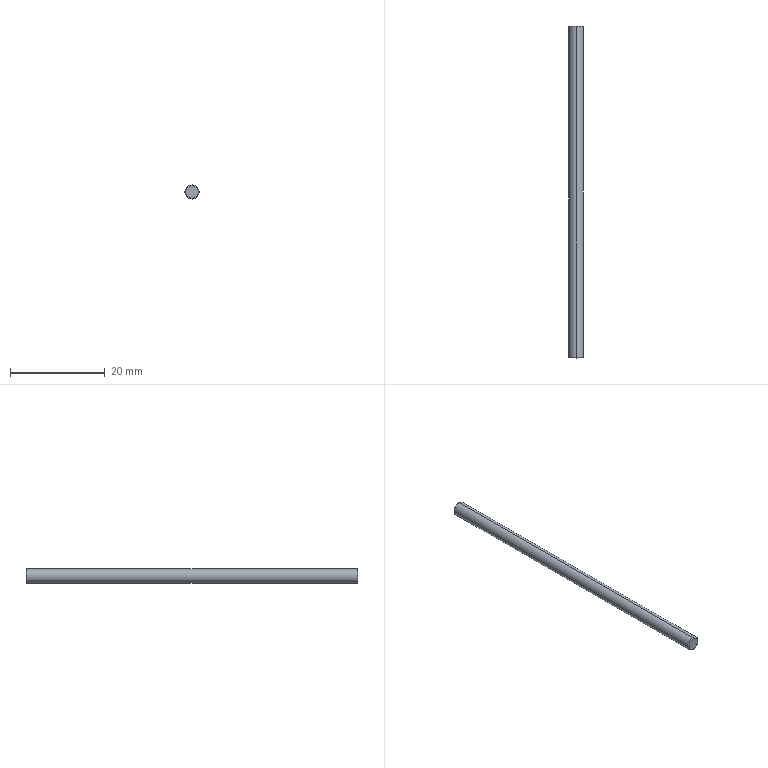Part | SolidWorks | features Extrusion 1, Fillet 1 | 1 solid | 8 faces | box 3 x 70 x 3 mm | volume 494.644 mm3 | torus 4 | cylinder 2 | plane 2 | commonest cylinder face diameters 3 x2
STEP:
#1=CARTESIAN_POINT('',(0.,69.8,-1.5));
#2=VERTEX_POINT('',#1);
#3=CARTESIAN_POINT('',(0.,69.8,1.5));
#4=VERTEX_POINT('',#3);
#5=CARTESIAN_POINT('',(0.,69.8,0.));
#6=DIRECTION('',(0.,-1.,0.));
#7=DIRECTION('',(0.,0.,1.));
#8=AXIS2_PLACEMENT_3D('',#5,#6,#7);
#9=CIRCLE('',#8,1.5);
#10=EDGE_CURVE('',#2,#4,#9,.T.);
#11=ORIENTED_EDGE('',*,*,#10,.F.);
#12=CARTESIAN_POINT('',(0.,70.,-1.3));
#13=VERTEX_POINT('',#12);
#14=CARTESIAN_POINT('',(0.,69.8,-1.3));
#15=DIRECTION('',(1.,0.,0.));
#16=DIRECTION('',(0.,0.,-1.));
#17=AXIS2_PLACEMENT_3D('',#14,#15,#16);
#18=CIRCLE('',#17,0.2);
#19=EDGE_CURVE('',#2,#13,#18,.T.);
#20=ORIENTED_EDGE('',*,*,#19,.T.);
#21=CARTESIAN_POINT('',(0.,70.,1.3));
#22=VERTEX_POINT('',#21);
#23=CARTESIAN_POINT('',(0.,70.,0.));
#24=DIRECTION('',(0.,1.,0.));
#25=DIRECTION('',(0.,0.,1.));
#26=AXIS2_PLACEMENT_3D('',#23,#24,#25);
#27=CIRCLE('',#26,1.3);
#28=EDGE_CURVE('',#22,#13,#27,.T.);
#29=ORIENTED_EDGE('',*,*,#28,.F.);
#30=CARTESIAN_POINT('',(0.,69.8,1.3));
#31=DIRECTION('',(-1.,0.,0.));
#32=DIRECTION('',(0.,0.,1.));
#33=AXIS2_PLACEMENT_3D('',#30,#31,#32);
#34=CIRCLE('',#33,0.2);
#35=EDGE_CURVE('',#4,#22,#34,.T.);
#36=ORIENTED_EDGE('',*,*,#35,.F.);
#37=EDGE_LOOP('',(#11,#20,#29,#36));
#38=FACE_OUTER_BOUND('',#37,.T.);
#39=CARTESIAN_POINT('',(0.,69.8,0.));
#40=DIRECTION('',(0.,1.,0.));
#41=DIRECTION('',(0.,0.,1.));
#42=AXIS2_PLACEMENT_3D('',#39,#40,#41);
#43=TOROIDAL_SURFACE('',#42,1.3,0.2);
#44=ADVANCED_FACE('',(#38),#43,.T.);
#45=CARTESIAN_POINT('',(0.,0.,-1.3));
#46=VERTEX_POINT('',#45);
#47=CARTESIAN_POINT('',(0.,0.,1.3));
#48=VERTEX_POINT('',#47);
#49=CARTESIAN_POINT('',(0.,0.,0.));
#50=DIRECTION('',(0.,-1.,0.));
#51=DIRECTION('',(0.,0.,1.));
#52=AXIS2_PLACEMENT_3D('',#49,#50,#51);
#53=CIRCLE('',#52,1.3);
#54=EDGE_CURVE('',#46,#48,#53,.T.);
#55=ORIENTED_EDGE('',*,*,#54,.F.);
#56=CARTESIAN_POINT('',(0.,0.2,-1.5));
#57=VERTEX_POINT('',#56);
#58=CARTESIAN_POINT('',(0.,0.2,-1.3));
#59=DIRECTION('',(1.,0.,0.));
#60=DIRECTION('',(0.,0.,-1.));
#61=AXIS2_PLACEMENT_3D('',#58,#59,#60);
#62=CIRCLE('',#61,0.2);
#63=EDGE_CURVE('',#46,#57,#62,.T.);
#64=ORIENTED_EDGE('',*,*,#63,.T.);
#65=CARTESIAN_POINT('',(0.,0.2,1.5));
#66=VERTEX_POINT('',#65);
#67=CARTESIAN_POINT('',(0.,0.2,0.));
#68=DIRECTION('',(0.,1.,0.));
#69=DIRECTION('',(0.,0.,1.));
#70=AXIS2_PLACEMENT_3D('',#67,#68,#69);
#71=CIRCLE('',#70,1.5);
#72=EDGE_CURVE('',#66,#57,#71,.T.);
#73=ORIENTED_EDGE('',*,*,#72,.F.);
#74=CARTESIAN_POINT('',(0.,0.2,1.3));
#75=DIRECTION('',(-1.,0.,0.));
#76=DIRECTION('',(0.,0.,1.));
#77=AXIS2_PLACEMENT_3D('',#74,#75,#76);
#78=CIRCLE('',#77,0.2);
#79=EDGE_CURVE('',#48,#66,#78,.T.);
#80=ORIENTED_EDGE('',*,*,#79,.F.);
#81=EDGE_LOOP('',(#55,#64,#73,#80));
#82=FACE_OUTER_BOUND('',#81,.T.);
#83=CARTESIAN_POINT('',(0.,0.2,0.));
#84=DIRECTION('',(0.,1.,0.));
#85=DIRECTION('',(0.,0.,1.));
#86=AXIS2_PLACEMENT_3D('',#83,#84,#85);
#87=TOROIDAL_SURFACE('',#86,1.3,0.2);
#88=ADVANCED_FACE('',(#82),#87,.T.);
#89=ORIENTED_EDGE('',*,*,#10,.T.);
#90=CARTESIAN_POINT('',(0.,70.,1.5));
#91=DIRECTION('',(0.,-1.,0.));
#92=VECTOR('',#91,1000.);
#93=LINE('',#90,#92);
#94=EDGE_CURVE('',#4,#66,#93,.T.);
#95=ORIENTED_EDGE('',*,*,#94,.T.);
#96=ORIENTED_EDGE('',*,*,#72,.T.);
#97=CARTESIAN_POINT('',(0.,70.,-1.5));
#98=DIRECTION('',(0.,-1.,0.));
#99=VECTOR('',#98,1000.);
#100=LINE('',#97,#99);
#101=EDGE_CURVE('',#2,#57,#100,.T.);
#102=ORIENTED_EDGE('',*,*,#101,.F.);
#103=EDGE_LOOP('',(#89,#95,#96,#102));
#104=FACE_OUTER_BOUND('',#103,.T.);
#105=CARTESIAN_POINT('',(0.,70.,0.));
#106=DIRECTION('',(0.,-1.,0.));
#107=DIRECTION('',(0.,0.,-1.));
#108=AXIS2_PLACEMENT_3D('',#105,#106,#107);
#109=CYLINDRICAL_SURFACE('',#108,1.5);
#110=ADVANCED_FACE('',(#104),#109,.T.);
#111=ORIENTED_EDGE('',*,*,#94,.F.);
#112=CARTESIAN_POINT('',(0.,69.8,0.));
#113=DIRECTION('',(0.,-1.,0.));
#114=DIRECTION('',(0.,0.,1.));
#115=AXIS2_PLACEMENT_3D('',#112,#113,#114);
#116=CIRCLE('',#115,1.5);
#117=EDGE_CURVE('',#4,#2,#116,.T.);
#118=ORIENTED_EDGE('',*,*,#117,.T.);
#119=ORIENTED_EDGE('',*,*,#101,.T.);
#120=CARTESIAN_POINT('',(0.,0.2,0.));
#121=DIRECTION('',(0.,1.,0.));
#122=DIRECTION('',(0.,0.,1.));
#123=AXIS2_PLACEMENT_3D('',#120,#121,#122);
#124=CIRCLE('',#123,1.5);
#125=EDGE_CURVE('',#57,#66,#124,.T.);
#126=ORIENTED_EDGE('',*,*,#125,.T.);
#127=EDGE_LOOP('',(#111,#118,#119,#126));
#128=FACE_OUTER_BOUND('',#127,.T.);
#129=CARTESIAN_POINT('',(0.,70.,0.));
#130=DIRECTION('',(0.,-1.,0.));
#131=DIRECTION('',(0.,0.,-1.));
#132=AXIS2_PLACEMENT_3D('',#129,#130,#131);
#133=CYLINDRICAL_SURFACE('',#132,1.5);
#134=ADVANCED_FACE('',(#128),#133,.T.);
#135=ORIENTED_EDGE('',*,*,#28,.T.);
#136=CARTESIAN_POINT('',(0.,70.,0.));
#137=DIRECTION('',(0.,1.,0.));
#138=DIRECTION('',(0.,0.,1.));
#139=AXIS2_PLACEMENT_3D('',#136,#137,#138);
#140=CIRCLE('',#139,1.3);
#141=EDGE_CURVE('',#13,#22,#140,.T.);
#142=ORIENTED_EDGE('',*,*,#141,.T.);
#143=EDGE_LOOP('',(#135,#142));
#144=FACE_OUTER_BOUND('',#143,.T.);
#145=CARTESIAN_POINT('',(0.,70.,0.));
#146=DIRECTION('',(0.,1.,0.));
#147=DIRECTION('',(0.,0.,1.));
#148=AXIS2_PLACEMENT_3D('',#145,#146,#147);
#149=PLANE('',#148);
#150=ADVANCED_FACE('',(#144),#149,.T.);
#151=CARTESIAN_POINT('',(0.,0.,0.));
#152=DIRECTION('',(0.,-1.,0.));
#153=DIRECTION('',(0.,0.,1.));
#154=AXIS2_PLACEMENT_3D('',#151,#152,#153);
#155=CIRCLE('',#154,1.3);
#156=EDGE_CURVE('',#48,#46,#155,.T.);
#157=ORIENTED_EDGE('',*,*,#156,.T.);
#158=ORIENTED_EDGE('',*,*,#54,.T.);
#159=EDGE_LOOP('',(#157,#158));
#160=FACE_OUTER_BOUND('',#159,.T.);
#161=CARTESIAN_POINT('',(0.,0.,0.));
#162=DIRECTION('',(0.,1.,0.));
#163=DIRECTION('',(0.,0.,1.));
#164=AXIS2_PLACEMENT_3D('',#161,#162,#163);
#165=PLANE('',#164);
#166=ADVANCED_FACE('',(#160),#165,.F.);
#167=ORIENTED_EDGE('',*,*,#63,.F.);
#168=ORIENTED_EDGE('',*,*,#156,.F.);
#169=ORIENTED_EDGE('',*,*,#79,.T.);
#170=ORIENTED_EDGE('',*,*,#125,.F.);
#171=EDGE_LOOP('',(#167,#168,#169,#170));
#172=FACE_OUTER_BOUND('',#171,.T.);
#173=CARTESIAN_POINT('',(0.,0.2,0.));
#174=DIRECTION('',(0.,1.,0.));
#175=DIRECTION('',(0.,0.,1.));
#176=AXIS2_PLACEMENT_3D('',#173,#174,#175);
#177=TOROIDAL_SURFACE('',#176,1.3,0.2);
#178=ADVANCED_FACE('',(#172),#177,.T.);
#179=ORIENTED_EDGE('',*,*,#19,.F.);
#180=ORIENTED_EDGE('',*,*,#117,.F.);
#181=ORIENTED_EDGE('',*,*,#35,.T.);
#182=ORIENTED_EDGE('',*,*,#141,.F.);
#183=EDGE_LOOP('',(#179,#180,#181,#182));
#184=FACE_OUTER_BOUND('',#183,.T.);
#185=CARTESIAN_POINT('',(0.,69.8,0.));
#186=DIRECTION('',(0.,1.,0.));
#187=DIRECTION('',(0.,0.,1.));
#188=AXIS2_PLACEMENT_3D('',#185,#186,#187);
#189=TOROIDAL_SURFACE('',#188,1.3,0.2);
#190=ADVANCED_FACE('',(#184),#189,.T.);
#191=CLOSED_SHELL('',(#44,#88,#110,#134,#150,#166,#178,#190));
#192=MANIFOLD_SOLID_BREP('',#191);
#193=CARTESIAN_POINT('',(0.,0.,0.));
#194=DIRECTION('',(0.,0.,1.));
#195=DIRECTION('',(1.,0.,0.));
#196=AXIS2_PLACEMENT_3D('',#193,#194,#195);
#197=(LENGTH_UNIT()NAMED_UNIT(*)SI_UNIT(.MILLI.,.METRE.));
#198=UNCERTAINTY_MEASURE_WITH_UNIT(LENGTH_MEASURE(0.00001),#197,'','');
#199=(NAMED_UNIT(*)PLANE_ANGLE_UNIT()SI_UNIT($,.RADIAN.));
#200=(NAMED_UNIT(*)SI_UNIT($,.STERADIAN.)SOLID_ANGLE_UNIT());
#201=(GEOMETRIC_REPRESENTATION_CONTEXT(3)GLOBAL_UNCERTAINTY_ASSIGNED_CONTEXT((#198))GLOBAL_UNIT_ASSIGNED_CONTEXT((#197,#199,#200))REPRESENTATION_CONTEXT('',''));
#202=ADVANCED_BREP_SHAPE_REPRESENTATION('',(#192,#196),#201);